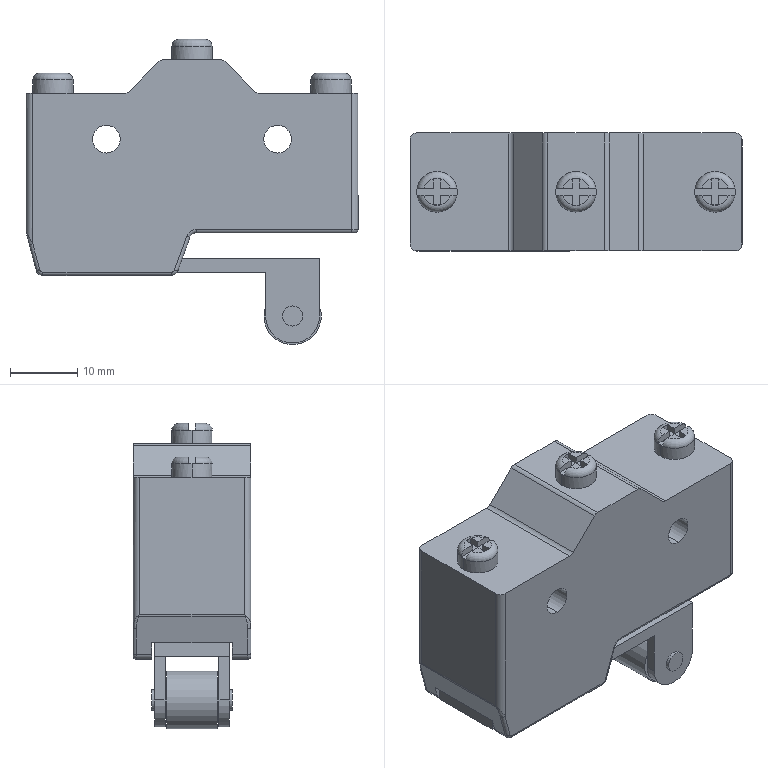Part | SolidWorks | features ICE 16, Chamfer 3, Fillet 3, Extrusion 1 | 1 solid | 670 faces | box 49.2 x 17.45 x 45.25 mm | volume 22167 mm3 | plane 431 | spline 180 | cylinder 45 | torus 14 | commonest cylinder face diameters 2 x14 1 x9 3 x8 6 x6 4.097 x4 8 x2